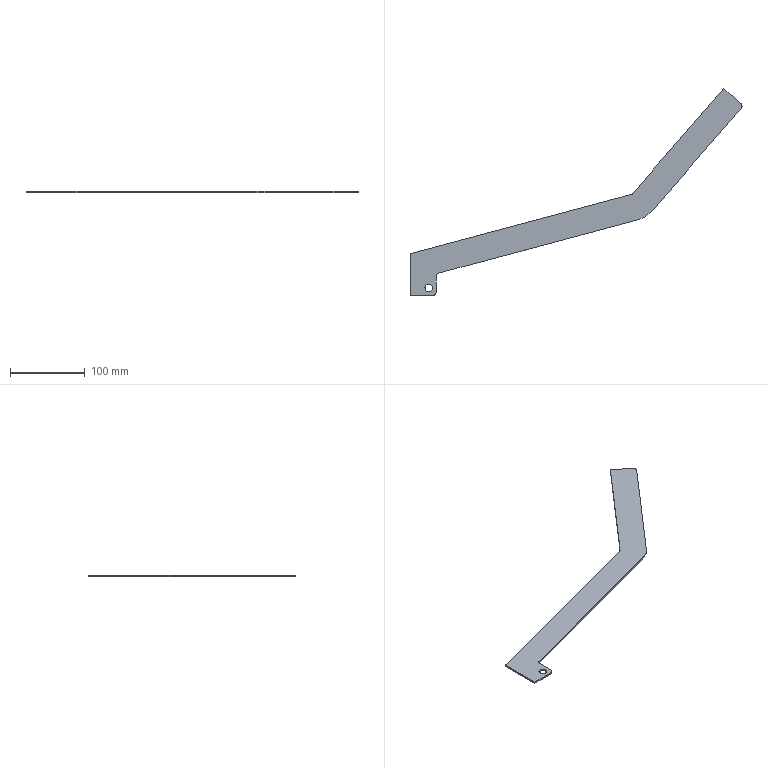Part | SolidWorks | features FlatPattern 1, SMBaseFlange 1, SheetMetal 1 | 1 solid | 19 faces | box 443.878 x 276.569 x 2.3 mm | volume 42757 mm3 | plane 10 | cylinder 9 | commonest cylinder face diameters 10 x6 2 x1 5 x1 72 x1
STEP:
#1=CARTESIAN_POINT('',(-1824.003,-308.367,-2.3));
#2=VERTEX_POINT('',#1);
#3=CARTESIAN_POINT('',(-1814.003,-308.367,-2.3));
#4=VERTEX_POINT('',#3);
#5=CARTESIAN_POINT('',(-1819.003,-308.367,-2.3));
#6=DIRECTION('',(0.,0.,1.));
#7=DIRECTION('',(1.,0.,0.));
#8=AXIS2_PLACEMENT_3D('',#5,#6,#7);
#9=CIRCLE('',#8,5.);
#10=EDGE_CURVE('',#2,#4,#9,.T.);
#11=ORIENTED_EDGE('',*,*,#10,.F.);
#12=CARTESIAN_POINT('',(-1824.003,-308.367,0.));
#13=VERTEX_POINT('',#12);
#14=CARTESIAN_POINT('',(-1824.003,-308.367,-2.3));
#15=DIRECTION('',(0.,0.,1.));
#16=VECTOR('',#15,1000.);
#17=LINE('',#14,#16);
#18=EDGE_CURVE('',#2,#13,#17,.T.);
#19=ORIENTED_EDGE('',*,*,#18,.T.);
#20=CARTESIAN_POINT('',(-1814.003,-308.367,0.));
#21=VERTEX_POINT('',#20);
#22=CARTESIAN_POINT('',(-1819.003,-308.367,0.));
#23=DIRECTION('',(0.,0.,1.));
#24=DIRECTION('',(1.,0.,0.));
#25=AXIS2_PLACEMENT_3D('',#22,#23,#24);
#26=CIRCLE('',#25,5.);
#27=EDGE_CURVE('',#13,#21,#26,.T.);
#28=ORIENTED_EDGE('',*,*,#27,.T.);
#29=CARTESIAN_POINT('',(-1814.003,-308.367,-2.3));
#30=DIRECTION('',(0.,0.,1.));
#31=VECTOR('',#30,1000.);
#32=LINE('',#29,#31);
#33=EDGE_CURVE('',#4,#21,#32,.T.);
#34=ORIENTED_EDGE('',*,*,#33,.F.);
#35=EDGE_LOOP('',(#11,#19,#28,#34));
#36=FACE_OUTER_BOUND('',#35,.T.);
#37=CARTESIAN_POINT('',(-1819.003,-308.367,-2.3));
#38=DIRECTION('',(0.,0.,1.));
#39=DIRECTION('',(1.,0.,0.));
#40=AXIS2_PLACEMENT_3D('',#37,#38,#39);
#41=CYLINDRICAL_SURFACE('',#40,5.);
#42=ADVANCED_FACE('',(#36),#41,.F.);
#43=CARTESIAN_POINT('',(-1401.351,-68.534,-2.3));
#44=VERTEX_POINT('',#43);
#45=CARTESIAN_POINT('',(-1400.125,-65.254,-2.3));
#46=VERTEX_POINT('',#45);
#47=CARTESIAN_POINT('',(-1405.125,-65.254,-2.3));
#48=DIRECTION('',(0.,0.,1.));
#49=DIRECTION('',(1.,0.,0.));
#50=AXIS2_PLACEMENT_3D('',#47,#48,#49);
#51=CIRCLE('',#50,5.);
#52=EDGE_CURVE('',#44,#46,#51,.T.);
#53=ORIENTED_EDGE('',*,*,#52,.T.);
#54=CARTESIAN_POINT('',(-1400.125,-65.254,0.));
#55=VERTEX_POINT('',#54);
#56=CARTESIAN_POINT('',(-1400.125,-65.254,-2.3));
#57=DIRECTION('',(0.,0.,1.));
#58=VECTOR('',#57,1000.);
#59=LINE('',#56,#58);
#60=EDGE_CURVE('',#46,#55,#59,.T.);
#61=ORIENTED_EDGE('',*,*,#60,.T.);
#62=CARTESIAN_POINT('',(-1401.351,-68.534,0.));
#63=VERTEX_POINT('',#62);
#64=CARTESIAN_POINT('',(-1405.125,-65.254,0.));
#65=DIRECTION('',(0.,0.,1.));
#66=DIRECTION('',(1.,0.,0.));
#67=AXIS2_PLACEMENT_3D('',#64,#65,#66);
#68=CIRCLE('',#67,5.);
#69=EDGE_CURVE('',#63,#55,#68,.T.);
#70=ORIENTED_EDGE('',*,*,#69,.F.);
#71=CARTESIAN_POINT('',(-1401.351,-68.534,-2.3));
#72=DIRECTION('',(0.,0.,1.));
#73=VECTOR('',#72,1000.);
#74=LINE('',#71,#73);
#75=EDGE_CURVE('',#44,#63,#74,.T.);
#76=ORIENTED_EDGE('',*,*,#75,.F.);
#77=EDGE_LOOP('',(#53,#61,#70,#76));
#78=FACE_OUTER_BOUND('',#77,.T.);
#79=CARTESIAN_POINT('',(-1405.125,-65.254,-2.3));
#80=DIRECTION('',(0.,0.,1.));
#81=DIRECTION('',(1.,0.,0.));
#82=AXIS2_PLACEMENT_3D('',#79,#80,#81);
#83=CYLINDRICAL_SURFACE('',#82,5.);
#84=ADVANCED_FACE('',(#78),#83,.T.);
#85=CARTESIAN_POINT('',(-1844.003,-318.367,0.));
#86=VERTEX_POINT('',#85);
#87=CARTESIAN_POINT('',(-1814.003,-318.367,0.));
#88=VERTEX_POINT('',#87);
#89=CARTESIAN_POINT('',(-1844.003,-318.367,0.));
#90=DIRECTION('',(1.,0.,0.));
#91=VECTOR('',#90,1000.);
#92=LINE('',#89,#91);
#93=EDGE_CURVE('',#86,#88,#92,.T.);
#94=ORIENTED_EDGE('',*,*,#93,.F.);
#95=CARTESIAN_POINT('',(-1844.003,-318.367,-2.3));
#96=VERTEX_POINT('',#95);
#97=CARTESIAN_POINT('',(-1844.003,-318.367,-2.3));
#98=DIRECTION('',(0.,0.,1.));
#99=VECTOR('',#98,1000.);
#100=LINE('',#97,#99);
#101=EDGE_CURVE('',#96,#86,#100,.T.);
#102=ORIENTED_EDGE('',*,*,#101,.F.);
#103=CARTESIAN_POINT('',(-1814.003,-318.367,-2.3));
#104=VERTEX_POINT('',#103);
#105=CARTESIAN_POINT('',(-1844.003,-318.367,-2.3));
#106=DIRECTION('',(1.,0.,0.));
#107=VECTOR('',#106,1000.);
#108=LINE('',#105,#107);
#109=EDGE_CURVE('',#96,#104,#108,.T.);
#110=ORIENTED_EDGE('',*,*,#109,.T.);
#111=CARTESIAN_POINT('',(-1814.003,-318.367,-2.3));
#112=DIRECTION('',(0.,0.,1.));
#113=VECTOR('',#112,1000.);
#114=LINE('',#111,#113);
#115=EDGE_CURVE('',#104,#88,#114,.T.);
#116=ORIENTED_EDGE('',*,*,#115,.T.);
#117=EDGE_LOOP('',(#94,#102,#110,#116));
#118=FACE_OUTER_BOUND('',#117,.T.);
#119=CARTESIAN_POINT('',(-1844.003,-318.367,-2.3));
#120=DIRECTION('',(0.,-1.,0.));
#121=DIRECTION('',(0.,0.,-1.));
#122=AXIS2_PLACEMENT_3D('',#119,#120,#121);
#123=PLANE('',#122);
#124=ADVANCED_FACE('',(#118),#123,.T.);
#125=CARTESIAN_POINT('',(-1844.003,-264.565,0.));
#126=VERTEX_POINT('',#125);
#127=CARTESIAN_POINT('',(-1844.003,-318.367,0.));
#128=DIRECTION('',(0.,-1.,0.));
#129=VECTOR('',#128,1000.);
#130=LINE('',#127,#129);
#131=EDGE_CURVE('',#126,#86,#130,.T.);
#132=ORIENTED_EDGE('',*,*,#131,.F.);
#133=CARTESIAN_POINT('',(-1844.003,-264.565,-2.3));
#134=VERTEX_POINT('',#133);
#135=CARTESIAN_POINT('',(-1844.003,-264.565,-2.3));
#136=DIRECTION('',(0.,0.,1.));
#137=VECTOR('',#136,1000.);
#138=LINE('',#135,#137);
#139=EDGE_CURVE('',#134,#126,#138,.T.);
#140=ORIENTED_EDGE('',*,*,#139,.F.);
#141=CARTESIAN_POINT('',(-1844.003,-318.367,-2.3));
#142=DIRECTION('',(0.,-1.,0.));
#143=VECTOR('',#142,1000.);
#144=LINE('',#141,#143);
#145=EDGE_CURVE('',#134,#96,#144,.T.);
#146=ORIENTED_EDGE('',*,*,#145,.T.);
#147=ORIENTED_EDGE('',*,*,#101,.T.);
#148=EDGE_LOOP('',(#132,#140,#146,#147));
#149=FACE_OUTER_BOUND('',#148,.T.);
#150=CARTESIAN_POINT('',(-1844.003,-318.367,-2.3));
#151=DIRECTION('',(-1.,0.,0.));
#152=DIRECTION('',(0.,0.,1.));
#153=AXIS2_PLACEMENT_3D('',#150,#151,#152);
#154=PLANE('',#153);
#155=ADVANCED_FACE('',(#149),#154,.T.);
#156=CARTESIAN_POINT('',(-1842.15,-262.15,0.));
#157=VERTEX_POINT('',#156);
#158=CARTESIAN_POINT('',(-1841.503,-264.565,0.));
#159=DIRECTION('',(0.,0.,1.));
#160=DIRECTION('',(-1.,0.,0.));
#161=AXIS2_PLACEMENT_3D('',#158,#159,#160);
#162=CIRCLE('',#161,2.5);
#163=EDGE_CURVE('',#157,#126,#162,.T.);
#164=ORIENTED_EDGE('',*,*,#163,.F.);
#165=CARTESIAN_POINT('',(-1842.15,-262.15,-2.3));
#166=VERTEX_POINT('',#165);
#167=CARTESIAN_POINT('',(-1842.15,-262.15,-2.3));
#168=DIRECTION('',(0.,0.,1.));
#169=VECTOR('',#168,1000.);
#170=LINE('',#167,#169);
#171=EDGE_CURVE('',#166,#157,#170,.T.);
#172=ORIENTED_EDGE('',*,*,#171,.F.);
#173=CARTESIAN_POINT('',(-1841.503,-264.565,-2.3));
#174=DIRECTION('',(0.,0.,1.));
#175=DIRECTION('',(-1.,0.,0.));
#176=AXIS2_PLACEMENT_3D('',#173,#174,#175);
#177=CIRCLE('',#176,2.5);
#178=EDGE_CURVE('',#166,#134,#177,.T.);
#179=ORIENTED_EDGE('',*,*,#178,.T.);
#180=ORIENTED_EDGE('',*,*,#139,.T.);
#181=EDGE_LOOP('',(#164,#172,#179,#180));
#182=FACE_OUTER_BOUND('',#181,.T.);
#183=CARTESIAN_POINT('',(-1841.503,-264.565,-2.3));
#184=DIRECTION('',(0.,0.,1.));
#185=DIRECTION('',(1.,0.,0.));
#186=AXIS2_PLACEMENT_3D('',#183,#184,#185);
#187=CYLINDRICAL_SURFACE('',#186,2.5);
#188=ADVANCED_FACE('',(#182),#187,.T.);
#189=CARTESIAN_POINT('',(-1547.669,-183.245,0.));
#190=VERTEX_POINT('',#189);
#191=CARTESIAN_POINT('',(-1842.15,-262.15,0.));
#192=DIRECTION('',(-0.9659,-0.2588,0.));
#193=VECTOR('',#192,1000.);
#194=LINE('',#191,#193);
#195=EDGE_CURVE('',#190,#157,#194,.T.);
#196=ORIENTED_EDGE('',*,*,#195,.F.);
#197=CARTESIAN_POINT('',(-1547.669,-183.245,-2.3));
#198=VERTEX_POINT('',#197);
#199=CARTESIAN_POINT('',(-1547.669,-183.245,-2.3));
#200=DIRECTION('',(0.,0.,1.));
#201=VECTOR('',#200,1000.);
#202=LINE('',#199,#201);
#203=EDGE_CURVE('',#198,#190,#202,.T.);
#204=ORIENTED_EDGE('',*,*,#203,.F.);
#205=CARTESIAN_POINT('',(-1842.15,-262.15,-2.3));
#206=DIRECTION('',(-0.9659,-0.2588,0.));
#207=VECTOR('',#206,1000.);
#208=LINE('',#205,#207);
#209=EDGE_CURVE('',#198,#166,#208,.T.);
#210=ORIENTED_EDGE('',*,*,#209,.T.);
#211=ORIENTED_EDGE('',*,*,#171,.T.);
#212=EDGE_LOOP('',(#196,#204,#210,#211));
#213=FACE_OUTER_BOUND('',#212,.T.);
#214=CARTESIAN_POINT('',(-1842.15,-262.15,-2.3));
#215=DIRECTION('',(-0.2588,0.9659,0.));
#216=DIRECTION('',(-0.9659,-0.2588,0.));
#217=AXIS2_PLACEMENT_3D('',#214,#215,#216);
#218=PLANE('',#217);
#219=ADVANCED_FACE('',(#213),#218,.T.);
#220=CARTESIAN_POINT('',(-1547.173,-182.935,0.));
#221=VERTEX_POINT('',#220);
#222=CARTESIAN_POINT('',(-1547.928,-182.279,0.));
#223=DIRECTION('',(0.,0.,-1.));
#224=DIRECTION('',(-1.,0.,0.));
#225=AXIS2_PLACEMENT_3D('',#222,#223,#224);
#226=CIRCLE('',#225,1.);
#227=EDGE_CURVE('',#221,#190,#226,.T.);
#228=ORIENTED_EDGE('',*,*,#227,.F.);
#229=CARTESIAN_POINT('',(-1547.173,-182.935,-2.3));
#230=VERTEX_POINT('',#229);
#231=CARTESIAN_POINT('',(-1547.173,-182.935,-2.3));
#232=DIRECTION('',(0.,0.,1.));
#233=VECTOR('',#232,1000.);
#234=LINE('',#231,#233);
#235=EDGE_CURVE('',#230,#221,#234,.T.);
#236=ORIENTED_EDGE('',*,*,#235,.F.);
#237=CARTESIAN_POINT('',(-1547.928,-182.279,-2.3));
#238=DIRECTION('',(0.,0.,-1.));
#239=DIRECTION('',(-1.,0.,0.));
#240=AXIS2_PLACEMENT_3D('',#237,#238,#239);
#241=CIRCLE('',#240,1.);
#242=EDGE_CURVE('',#230,#198,#241,.T.);
#243=ORIENTED_EDGE('',*,*,#242,.T.);
#244=ORIENTED_EDGE('',*,*,#203,.T.);
#245=EDGE_LOOP('',(#228,#236,#243,#244));
#246=FACE_OUTER_BOUND('',#245,.T.);
#247=CARTESIAN_POINT('',(-1547.928,-182.279,-2.3));
#248=DIRECTION('',(0.,0.,1.));
#249=DIRECTION('',(1.,0.,0.));
#250=AXIS2_PLACEMENT_3D('',#247,#248,#249);
#251=CYLINDRICAL_SURFACE('',#250,1.);
#252=ADVANCED_FACE('',(#246),#251,.F.);
#253=CARTESIAN_POINT('',(-1424.486,-41.799,0.));
#254=VERTEX_POINT('',#253);
#255=CARTESIAN_POINT('',(-1547.173,-182.935,0.));
#256=DIRECTION('',(-0.6561,-0.7547,0.));
#257=VECTOR('',#256,1000.);
#258=LINE('',#255,#257);
#259=EDGE_CURVE('',#254,#221,#258,.T.);
#260=ORIENTED_EDGE('',*,*,#259,.F.);
#261=CARTESIAN_POINT('',(-1424.486,-41.799,-2.3));
#262=VERTEX_POINT('',#261);
#263=CARTESIAN_POINT('',(-1424.486,-41.799,-2.3));
#264=DIRECTION('',(0.,0.,1.));
#265=VECTOR('',#264,1000.);
#266=LINE('',#263,#265);
#267=EDGE_CURVE('',#262,#254,#266,.T.);
#268=ORIENTED_EDGE('',*,*,#267,.F.);
#269=CARTESIAN_POINT('',(-1547.173,-182.935,-2.3));
#270=DIRECTION('',(-0.6561,-0.7547,0.));
#271=VECTOR('',#270,1000.);
#272=LINE('',#269,#271);
#273=EDGE_CURVE('',#262,#230,#272,.T.);
#274=ORIENTED_EDGE('',*,*,#273,.T.);
#275=ORIENTED_EDGE('',*,*,#235,.T.);
#276=EDGE_LOOP('',(#260,#268,#274,#275));
#277=FACE_OUTER_BOUND('',#276,.T.);
#278=CARTESIAN_POINT('',(-1547.173,-182.935,-2.3));
#279=DIRECTION('',(-0.7547,0.6561,0.));
#280=DIRECTION('',(-0.6561,-0.7547,0.));
#281=AXIS2_PLACEMENT_3D('',#278,#279,#280);
#282=PLANE('',#281);
#283=ADVANCED_FACE('',(#277),#282,.T.);
#284=CARTESIAN_POINT('',(-1401.844,-61.48,0.));
#285=VERTEX_POINT('',#284);
#286=CARTESIAN_POINT('',(-1424.486,-41.799,0.));
#287=DIRECTION('',(-0.7547,0.6561,0.));
#288=VECTOR('',#287,1000.);
#289=LINE('',#286,#288);
#290=EDGE_CURVE('',#285,#254,#289,.T.);
#291=ORIENTED_EDGE('',*,*,#290,.F.);
#292=CARTESIAN_POINT('',(-1401.844,-61.48,-2.3));
#293=VERTEX_POINT('',#292);
#294=CARTESIAN_POINT('',(-1401.844,-61.48,-2.3));
#295=DIRECTION('',(0.,0.,1.));
#296=VECTOR('',#295,1000.);
#297=LINE('',#294,#296);
#298=EDGE_CURVE('',#293,#285,#297,.T.);
#299=ORIENTED_EDGE('',*,*,#298,.F.);
#300=CARTESIAN_POINT('',(-1424.486,-41.799,-2.3));
#301=DIRECTION('',(-0.7547,0.6561,0.));
#302=VECTOR('',#301,1000.);
#303=LINE('',#300,#302);
#304=EDGE_CURVE('',#293,#262,#303,.T.);
#305=ORIENTED_EDGE('',*,*,#304,.T.);
#306=ORIENTED_EDGE('',*,*,#267,.T.);
#307=EDGE_LOOP('',(#291,#299,#305,#306));
#308=FACE_OUTER_BOUND('',#307,.T.);
#309=CARTESIAN_POINT('',(-1424.486,-41.799,-2.3));
#310=DIRECTION('',(0.6561,0.7547,0.));
#311=DIRECTION('',(-0.7547,0.6561,0.));
#312=AXIS2_PLACEMENT_3D('',#309,#310,#311);
#313=PLANE('',#312);
#314=ADVANCED_FACE('',(#308),#313,.T.);
#315=ORIENTED_EDGE('',*,*,#60,.F.);
#316=CARTESIAN_POINT('',(-1405.125,-65.254,-2.3));
#317=DIRECTION('',(0.,0.,1.));
#318=DIRECTION('',(1.,0.,0.));
#319=AXIS2_PLACEMENT_3D('',#316,#317,#318);
#320=CIRCLE('',#319,5.);
#321=EDGE_CURVE('',#46,#293,#320,.T.);
#322=ORIENTED_EDGE('',*,*,#321,.T.);
#323=ORIENTED_EDGE('',*,*,#298,.T.);
#324=CARTESIAN_POINT('',(-1405.125,-65.254,0.));
#325=DIRECTION('',(0.,0.,1.));
#326=DIRECTION('',(1.,0.,0.));
#327=AXIS2_PLACEMENT_3D('',#324,#325,#326);
#328=CIRCLE('',#327,5.);
#329=EDGE_CURVE('',#55,#285,#328,.T.);
#330=ORIENTED_EDGE('',*,*,#329,.F.);
#331=EDGE_LOOP('',(#315,#322,#323,#330));
#332=FACE_OUTER_BOUND('',#331,.T.);
#333=CARTESIAN_POINT('',(-1405.125,-65.254,-2.3));
#334=DIRECTION('',(0.,0.,1.));
#335=DIRECTION('',(1.,0.,0.));
#336=AXIS2_PLACEMENT_3D('',#333,#334,#335);
#337=CYLINDRICAL_SURFACE('',#336,5.);
#338=ADVANCED_FACE('',(#332),#337,.T.);
#339=CARTESIAN_POINT('',(-1520.759,-205.897,0.));
#340=VERTEX_POINT('',#339);
#341=CARTESIAN_POINT('',(-1520.759,-205.897,0.));
#342=DIRECTION('',(0.6561,0.7547,0.));
#343=VECTOR('',#342,1000.);
#344=LINE('',#341,#343);
#345=EDGE_CURVE('',#340,#63,#344,.T.);
#346=ORIENTED_EDGE('',*,*,#345,.F.);
#347=CARTESIAN_POINT('',(-1520.759,-205.897,-2.3));
#348=VERTEX_POINT('',#347);
#349=CARTESIAN_POINT('',(-1520.759,-205.897,-2.3));
#350=DIRECTION('',(0.,0.,1.));
#351=VECTOR('',#350,1000.);
#352=LINE('',#349,#351);
#353=EDGE_CURVE('',#348,#340,#352,.T.);
#354=ORIENTED_EDGE('',*,*,#353,.F.);
#355=CARTESIAN_POINT('',(-1520.759,-205.897,-2.3));
#356=DIRECTION('',(0.6561,0.7547,0.));
#357=VECTOR('',#356,1000.);
#358=LINE('',#355,#357);
#359=EDGE_CURVE('',#348,#44,#358,.T.);
#360=ORIENTED_EDGE('',*,*,#359,.T.);
#361=ORIENTED_EDGE('',*,*,#75,.T.);
#362=EDGE_LOOP('',(#346,#354,#360,#361));
#363=FACE_OUTER_BOUND('',#362,.T.);
#364=CARTESIAN_POINT('',(-1520.759,-205.897,-2.3));
#365=DIRECTION('',(0.7547,-0.6561,0.));
#366=DIRECTION('',(0.6561,0.7547,0.));
#367=AXIS2_PLACEMENT_3D('',#364,#365,#366);
#368=PLANE('',#367);
#369=ADVANCED_FACE('',(#363),#368,.T.);
#370=CARTESIAN_POINT('',(-1538.611,-217.052,0.));
#371=VERTEX_POINT('',#370);
#372=CARTESIAN_POINT('',(-1547.928,-182.279,0.));
#373=DIRECTION('',(0.,0.,1.));
#374=DIRECTION('',(-1.,0.,0.));
#375=AXIS2_PLACEMENT_3D('',#372,#373,#374);
#376=CIRCLE('',#375,36.);
#377=EDGE_CURVE('',#371,#340,#376,.T.);
#378=ORIENTED_EDGE('',*,*,#377,.F.);
#379=CARTESIAN_POINT('',(-1538.611,-217.052,-2.3));
#380=VERTEX_POINT('',#379);
#381=CARTESIAN_POINT('',(-1538.611,-217.052,-2.3));
#382=DIRECTION('',(0.,0.,1.));
#383=VECTOR('',#382,1000.);
#384=LINE('',#381,#383);
#385=EDGE_CURVE('',#380,#371,#384,.T.);
#386=ORIENTED_EDGE('',*,*,#385,.F.);
#387=CARTESIAN_POINT('',(-1547.928,-182.279,-2.3));
#388=DIRECTION('',(0.,0.,1.));
#389=DIRECTION('',(-1.,0.,0.));
#390=AXIS2_PLACEMENT_3D('',#387,#388,#389);
#391=CIRCLE('',#390,36.);
#392=EDGE_CURVE('',#380,#348,#391,.T.);
#393=ORIENTED_EDGE('',*,*,#392,.T.);
#394=ORIENTED_EDGE('',*,*,#353,.T.);
#395=EDGE_LOOP('',(#378,#386,#393,#394));
#396=FACE_OUTER_BOUND('',#395,.T.);
#397=CARTESIAN_POINT('',(-1547.928,-182.279,-2.3));
#398=DIRECTION('',(0.,0.,1.));
#399=DIRECTION('',(1.,0.,0.));
#400=AXIS2_PLACEMENT_3D('',#397,#398,#399);
#401=CYLINDRICAL_SURFACE('',#400,36.);
#402=ADVANCED_FACE('',(#396),#401,.T.);
#403=CARTESIAN_POINT('',(-1805.297,-288.51,0.));
#404=VERTEX_POINT('',#403);
#405=CARTESIAN_POINT('',(-1805.297,-288.51,0.));
#406=DIRECTION('',(0.9659,0.2588,0.));
#407=VECTOR('',#406,1000.);
#408=LINE('',#405,#407);
#409=EDGE_CURVE('',#404,#371,#408,.T.);
#410=ORIENTED_EDGE('',*,*,#409,.F.);
#411=CARTESIAN_POINT('',(-1805.297,-288.51,-2.3));
#412=VERTEX_POINT('',#411);
#413=CARTESIAN_POINT('',(-1805.297,-288.51,-2.3));
#414=DIRECTION('',(0.,0.,1.));
#415=VECTOR('',#414,1000.);
#416=LINE('',#413,#415);
#417=EDGE_CURVE('',#412,#404,#416,.T.);
#418=ORIENTED_EDGE('',*,*,#417,.F.);
#419=CARTESIAN_POINT('',(-1805.297,-288.51,-2.3));
#420=DIRECTION('',(0.9659,0.2588,0.));
#421=VECTOR('',#420,1000.);
#422=LINE('',#419,#421);
#423=EDGE_CURVE('',#412,#380,#422,.T.);
#424=ORIENTED_EDGE('',*,*,#423,.T.);
#425=ORIENTED_EDGE('',*,*,#385,.T.);
#426=EDGE_LOOP('',(#410,#418,#424,#425));
#427=FACE_OUTER_BOUND('',#426,.T.);
#428=CARTESIAN_POINT('',(-1805.297,-288.51,-2.3));
#429=DIRECTION('',(0.2588,-0.9659,0.));
#430=DIRECTION('',(0.9659,0.2588,0.));
#431=AXIS2_PLACEMENT_3D('',#428,#429,#430);
#432=PLANE('',#431);
#433=ADVANCED_FACE('',(#427),#432,.T.);
#434=CARTESIAN_POINT('',(-1809.003,-293.34,0.));
#435=VERTEX_POINT('',#434);
#436=CARTESIAN_POINT('',(-1804.003,-293.34,0.));
#437=DIRECTION('',(0.,0.,-1.));
#438=DIRECTION('',(-1.,0.,0.));
#439=AXIS2_PLACEMENT_3D('',#436,#437,#438);
#440=CIRCLE('',#439,5.);
#441=EDGE_CURVE('',#435,#404,#440,.T.);
#442=ORIENTED_EDGE('',*,*,#441,.F.);
#443=CARTESIAN_POINT('',(-1809.003,-293.34,-2.3));
#444=VERTEX_POINT('',#443);
#445=CARTESIAN_POINT('',(-1809.003,-293.34,-2.3));
#446=DIRECTION('',(0.,0.,1.));
#447=VECTOR('',#446,1000.);
#448=LINE('',#445,#447);
#449=EDGE_CURVE('',#444,#435,#448,.T.);
#450=ORIENTED_EDGE('',*,*,#449,.F.);
#451=CARTESIAN_POINT('',(-1804.003,-293.34,-2.3));
#452=DIRECTION('',(0.,0.,-1.));
#453=DIRECTION('',(-1.,0.,0.));
#454=AXIS2_PLACEMENT_3D('',#451,#452,#453);
#455=CIRCLE('',#454,5.);
#456=EDGE_CURVE('',#444,#412,#455,.T.);
#457=ORIENTED_EDGE('',*,*,#456,.T.);
#458=ORIENTED_EDGE('',*,*,#417,.T.);
#459=EDGE_LOOP('',(#442,#450,#457,#458));
#460=FACE_OUTER_BOUND('',#459,.T.);
#461=CARTESIAN_POINT('',(-1804.003,-293.34,-2.3));
#462=DIRECTION('',(0.,0.,1.));
#463=DIRECTION('',(1.,0.,0.));
#464=AXIS2_PLACEMENT_3D('',#461,#462,#463);
#465=CYLINDRICAL_SURFACE('',#464,5.);
#466=ADVANCED_FACE('',(#460),#465,.F.);
#467=CARTESIAN_POINT('',(-1809.003,-313.367,0.));
#468=VERTEX_POINT('',#467);
#469=CARTESIAN_POINT('',(-1809.003,-313.367,0.));
#470=DIRECTION('',(0.,1.,0.));
#471=VECTOR('',#470,1000.);
#472=LINE('',#469,#471);
#473=EDGE_CURVE('',#468,#435,#472,.T.);
#474=ORIENTED_EDGE('',*,*,#473,.F.);
#475=CARTESIAN_POINT('',(-1809.003,-313.367,-2.3));
#476=VERTEX_POINT('',#475);
#477=CARTESIAN_POINT('',(-1809.003,-313.367,-2.3));
#478=DIRECTION('',(0.,0.,1.));
#479=VECTOR('',#478,1000.);
#480=LINE('',#477,#479);
#481=EDGE_CURVE('',#476,#468,#480,.T.);
#482=ORIENTED_EDGE('',*,*,#481,.F.);
#483=CARTESIAN_POINT('',(-1809.003,-313.367,-2.3));
#484=DIRECTION('',(0.,1.,0.));
#485=VECTOR('',#484,1000.);
#486=LINE('',#483,#485);
#487=EDGE_CURVE('',#476,#444,#486,.T.);
#488=ORIENTED_EDGE('',*,*,#487,.T.);
#489=ORIENTED_EDGE('',*,*,#449,.T.);
#490=EDGE_LOOP('',(#474,#482,#488,#489));
#491=FACE_OUTER_BOUND('',#490,.T.);
#492=CARTESIAN_POINT('',(-1809.003,-313.367,-2.3));
#493=DIRECTION('',(1.,0.,0.));
#494=DIRECTION('',(0.,1.,0.));
#495=AXIS2_PLACEMENT_3D('',#492,#493,#494);
#496=PLANE('',#495);
#497=ADVANCED_FACE('',(#491),#496,.T.);
#498=CARTESIAN_POINT('',(-1814.003,-313.367,0.));
#499=DIRECTION('',(0.,0.,1.));
#500=DIRECTION('',(1.,0.,0.));
#501=AXIS2_PLACEMENT_3D('',#498,#499,#500);
#502=CIRCLE('',#501,5.);
#503=EDGE_CURVE('',#88,#468,#502,.T.);
#504=ORIENTED_EDGE('',*,*,#503,.F.);
#505=ORIENTED_EDGE('',*,*,#115,.F.);
#506=CARTESIAN_POINT('',(-1814.003,-313.367,-2.3));
#507=DIRECTION('',(0.,0.,1.));
#508=DIRECTION('',(1.,0.,0.));
#509=AXIS2_PLACEMENT_3D('',#506,#507,#508);
#510=CIRCLE('',#509,5.);
#511=EDGE_CURVE('',#104,#476,#510,.T.);
#512=ORIENTED_EDGE('',*,*,#511,.T.);
#513=ORIENTED_EDGE('',*,*,#481,.T.);
#514=EDGE_LOOP('',(#504,#505,#512,#513));
#515=FACE_OUTER_BOUND('',#514,.T.);
#516=CARTESIAN_POINT('',(-1814.003,-313.367,-2.3));
#517=DIRECTION('',(0.,0.,1.));
#518=DIRECTION('',(1.,0.,0.));
#519=AXIS2_PLACEMENT_3D('',#516,#517,#518);
#520=CYLINDRICAL_SURFACE('',#519,5.);
#521=ADVANCED_FACE('',(#515),#520,.T.);
#522=CARTESIAN_POINT('',(-1819.003,-308.367,-2.3));
#523=DIRECTION('',(0.,0.,1.));
#524=DIRECTION('',(1.,0.,0.));
#525=AXIS2_PLACEMENT_3D('',#522,#523,#524);
#526=CIRCLE('',#525,5.);
#527=EDGE_CURVE('',#4,#2,#526,.T.);
#528=ORIENTED_EDGE('',*,*,#527,.T.);
#529=ORIENTED_EDGE('',*,*,#10,.T.);
#530=EDGE_LOOP('',(#528,#529));
#531=FACE_BOUND('',#530,.T.);
#532=ORIENTED_EDGE('',*,*,#109,.F.);
#533=ORIENTED_EDGE('',*,*,#145,.F.);
#534=ORIENTED_EDGE('',*,*,#178,.F.);
#535=ORIENTED_EDGE('',*,*,#209,.F.);
#536=ORIENTED_EDGE('',*,*,#242,.F.);
#537=ORIENTED_EDGE('',*,*,#273,.F.);
#538=ORIENTED_EDGE('',*,*,#304,.F.);
#539=ORIENTED_EDGE('',*,*,#321,.F.);
#540=ORIENTED_EDGE('',*,*,#52,.F.);
#541=ORIENTED_EDGE('',*,*,#359,.F.);
#542=ORIENTED_EDGE('',*,*,#392,.F.);
#543=ORIENTED_EDGE('',*,*,#423,.F.);
#544=ORIENTED_EDGE('',*,*,#456,.F.);
#545=ORIENTED_EDGE('',*,*,#487,.F.);
#546=ORIENTED_EDGE('',*,*,#511,.F.);
#547=EDGE_LOOP('',(#532,#533,#534,#535,#536,#537,#538,#539,#540,#541,#542,#543,#544,#545,#546));
#548=FACE_OUTER_BOUND('',#547,.T.);
#549=CARTESIAN_POINT('',(-1814.003,-313.367,-2.3));
#550=DIRECTION('',(0.,0.,1.));
#551=DIRECTION('',(1.,0.,0.));
#552=AXIS2_PLACEMENT_3D('',#549,#550,#551);
#553=PLANE('',#552);
#554=ADVANCED_FACE('',(#531,#548),#553,.F.);
#555=CARTESIAN_POINT('',(-1819.003,-308.367,0.));
#556=DIRECTION('',(0.,0.,1.));
#557=DIRECTION('',(1.,0.,0.));
#558=AXIS2_PLACEMENT_3D('',#555,#556,#557);
#559=CIRCLE('',#558,5.);
#560=EDGE_CURVE('',#21,#13,#559,.T.);
#561=ORIENTED_EDGE('',*,*,#560,.F.);
#562=ORIENTED_EDGE('',*,*,#27,.F.);
#563=EDGE_LOOP('',(#561,#562));
#564=FACE_BOUND('',#563,.T.);
#565=ORIENTED_EDGE('',*,*,#93,.T.);
#566=ORIENTED_EDGE('',*,*,#503,.T.);
#567=ORIENTED_EDGE('',*,*,#473,.T.);
#568=ORIENTED_EDGE('',*,*,#441,.T.);
#569=ORIENTED_EDGE('',*,*,#409,.T.);
#570=ORIENTED_EDGE('',*,*,#377,.T.);
#571=ORIENTED_EDGE('',*,*,#345,.T.);
#572=ORIENTED_EDGE('',*,*,#69,.T.);
#573=ORIENTED_EDGE('',*,*,#329,.T.);
#574=ORIENTED_EDGE('',*,*,#290,.T.);
#575=ORIENTED_EDGE('',*,*,#259,.T.);
#576=ORIENTED_EDGE('',*,*,#227,.T.);
#577=ORIENTED_EDGE('',*,*,#195,.T.);
#578=ORIENTED_EDGE('',*,*,#163,.T.);
#579=ORIENTED_EDGE('',*,*,#131,.T.);
#580=EDGE_LOOP('',(#565,#566,#567,#568,#569,#570,#571,#572,#573,#574,#575,#576,#577,#578,#579));
#581=FACE_OUTER_BOUND('',#580,.T.);
#582=CARTESIAN_POINT('',(-1814.003,-313.367,0.));
#583=DIRECTION('',(0.,0.,1.));
#584=DIRECTION('',(1.,0.,0.));
#585=AXIS2_PLACEMENT_3D('',#582,#583,#584);
#586=PLANE('',#585);
#587=ADVANCED_FACE('',(#564,#581),#586,.T.);
#588=ORIENTED_EDGE('',*,*,#18,.F.);
#589=ORIENTED_EDGE('',*,*,#527,.F.);
#590=ORIENTED_EDGE('',*,*,#33,.T.);
#591=ORIENTED_EDGE('',*,*,#560,.T.);
#592=EDGE_LOOP('',(#588,#589,#590,#591));
#593=FACE_OUTER_BOUND('',#592,.T.);
#594=CARTESIAN_POINT('',(-1819.003,-308.367,-2.3));
#595=DIRECTION('',(0.,0.,1.));
#596=DIRECTION('',(1.,0.,0.));
#597=AXIS2_PLACEMENT_3D('',#594,#595,#596);
#598=CYLINDRICAL_SURFACE('',#597,5.);
#599=ADVANCED_FACE('',(#593),#598,.F.);
#600=CLOSED_SHELL('',(#42,#84,#124,#155,#188,#219,#252,#283,#314,#338,#369,#402,#433,#466,#497,#521,#554,#587,#599));
#601=MANIFOLD_SOLID_BREP('',#600);
#602=CARTESIAN_POINT('',(0.,0.,0.));
#603=DIRECTION('',(0.,0.,1.));
#604=DIRECTION('',(1.,0.,0.));
#605=AXIS2_PLACEMENT_3D('',#602,#603,#604);
#606=(LENGTH_UNIT()NAMED_UNIT(*)SI_UNIT(.MILLI.,.METRE.));
#607=UNCERTAINTY_MEASURE_WITH_UNIT(LENGTH_MEASURE(0.00001),#606,'','');
#608=(NAMED_UNIT(*)PLANE_ANGLE_UNIT()SI_UNIT($,.RADIAN.));
#609=(NAMED_UNIT(*)SI_UNIT($,.STERADIAN.)SOLID_ANGLE_UNIT());
#610=(GEOMETRIC_REPRESENTATION_CONTEXT(3)GLOBAL_UNCERTAINTY_ASSIGNED_CONTEXT((#607))GLOBAL_UNIT_ASSIGNED_CONTEXT((#606,#608,#609))REPRESENTATION_CONTEXT('',''));
#611=ADVANCED_BREP_SHAPE_REPRESENTATION('',(#601,#605),#610);